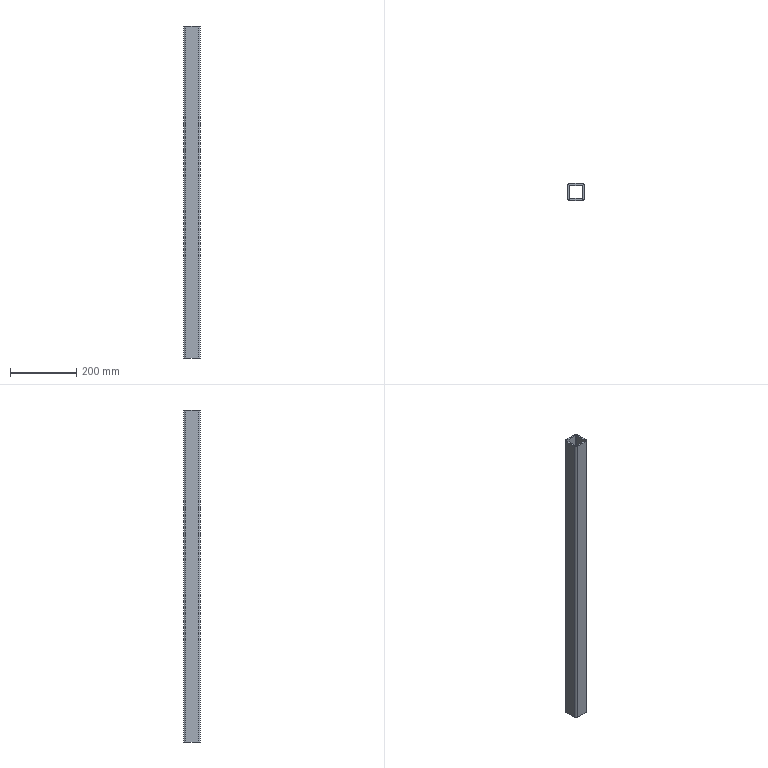Part | SolidWorks | features Extrusion 1 | 1 solid | 18 faces | box 50 x 50 x 1000 mm | volume 869956 mm3 | plane 10 | cylinder 8 | commonest cylinder face diameters 2 x4 12 x4
STEP:
#1=CARTESIAN_POINT('',(0.,6.,1000.));
#2=VERTEX_POINT('',#1);
#3=CARTESIAN_POINT('',(6.,0.,1000.));
#4=VERTEX_POINT('',#3);
#5=CARTESIAN_POINT('',(6.,6.,1000.));
#6=DIRECTION('',(0.,0.,1.));
#7=DIRECTION('',(-1.,0.,0.));
#8=AXIS2_PLACEMENT_3D('',#5,#6,#7);
#9=CIRCLE('',#8,6.);
#10=EDGE_CURVE('',#2,#4,#9,.T.);
#11=ORIENTED_EDGE('',*,*,#10,.T.);
#12=CARTESIAN_POINT('',(44.,0.,1000.));
#13=VERTEX_POINT('',#12);
#14=CARTESIAN_POINT('',(6.,0.,1000.));
#15=DIRECTION('',(1.,0.,0.));
#16=VECTOR('',#15,1000.);
#17=LINE('',#14,#16);
#18=EDGE_CURVE('',#4,#13,#17,.T.);
#19=ORIENTED_EDGE('',*,*,#18,.T.);
#20=CARTESIAN_POINT('',(50.,6.,1000.));
#21=VERTEX_POINT('',#20);
#22=CARTESIAN_POINT('',(44.,6.,1000.));
#23=DIRECTION('',(0.,0.,1.));
#24=DIRECTION('',(1.,0.,0.));
#25=AXIS2_PLACEMENT_3D('',#22,#23,#24);
#26=CIRCLE('',#25,6.);
#27=EDGE_CURVE('',#13,#21,#26,.T.);
#28=ORIENTED_EDGE('',*,*,#27,.T.);
#29=CARTESIAN_POINT('',(50.,44.,1000.));
#30=VERTEX_POINT('',#29);
#31=CARTESIAN_POINT('',(50.,6.,1000.));
#32=DIRECTION('',(0.,1.,0.));
#33=VECTOR('',#32,1000.);
#34=LINE('',#31,#33);
#35=EDGE_CURVE('',#21,#30,#34,.T.);
#36=ORIENTED_EDGE('',*,*,#35,.T.);
#37=CARTESIAN_POINT('',(44.,50.,1000.));
#38=VERTEX_POINT('',#37);
#39=CARTESIAN_POINT('',(44.,44.,1000.));
#40=DIRECTION('',(0.,0.,1.));
#41=DIRECTION('',(-1.,0.,0.));
#42=AXIS2_PLACEMENT_3D('',#39,#40,#41);
#43=CIRCLE('',#42,6.);
#44=EDGE_CURVE('',#30,#38,#43,.T.);
#45=ORIENTED_EDGE('',*,*,#44,.T.);
#46=CARTESIAN_POINT('',(6.,50.,1000.));
#47=VERTEX_POINT('',#46);
#48=CARTESIAN_POINT('',(6.,50.,1000.));
#49=DIRECTION('',(-1.,0.,0.));
#50=VECTOR('',#49,1000.);
#51=LINE('',#48,#50);
#52=EDGE_CURVE('',#38,#47,#51,.T.);
#53=ORIENTED_EDGE('',*,*,#52,.T.);
#54=CARTESIAN_POINT('',(0.,44.,1000.));
#55=VERTEX_POINT('',#54);
#56=CARTESIAN_POINT('',(6.,44.,1000.));
#57=DIRECTION('',(0.,0.,1.));
#58=DIRECTION('',(-1.,0.,0.));
#59=AXIS2_PLACEMENT_3D('',#56,#57,#58);
#60=CIRCLE('',#59,6.);
#61=EDGE_CURVE('',#47,#55,#60,.T.);
#62=ORIENTED_EDGE('',*,*,#61,.T.);
#63=CARTESIAN_POINT('',(0.,6.,1000.));
#64=DIRECTION('',(0.,-1.,0.));
#65=VECTOR('',#64,1000.);
#66=LINE('',#63,#65);
#67=EDGE_CURVE('',#55,#2,#66,.T.);
#68=ORIENTED_EDGE('',*,*,#67,.T.);
#69=EDGE_LOOP('',(#11,#19,#28,#36,#45,#53,#62,#68));
#70=FACE_OUTER_BOUND('',#69,.T.);
#71=CARTESIAN_POINT('',(6.,45.,1000.));
#72=VERTEX_POINT('',#71);
#73=CARTESIAN_POINT('',(5.,44.,1000.));
#74=VERTEX_POINT('',#73);
#75=CARTESIAN_POINT('',(6.,44.,1000.));
#76=DIRECTION('',(0.,0.,1.));
#77=DIRECTION('',(-1.,0.,0.));
#78=AXIS2_PLACEMENT_3D('',#75,#76,#77);
#79=CIRCLE('',#78,1.);
#80=EDGE_CURVE('',#72,#74,#79,.T.);
#81=ORIENTED_EDGE('',*,*,#80,.F.);
#82=CARTESIAN_POINT('',(44.,45.,1000.));
#83=VERTEX_POINT('',#82);
#84=CARTESIAN_POINT('',(6.,45.,1000.));
#85=DIRECTION('',(-1.,0.,0.));
#86=VECTOR('',#85,1000.);
#87=LINE('',#84,#86);
#88=EDGE_CURVE('',#83,#72,#87,.T.);
#89=ORIENTED_EDGE('',*,*,#88,.F.);
#90=CARTESIAN_POINT('',(45.,44.,1000.));
#91=VERTEX_POINT('',#90);
#92=CARTESIAN_POINT('',(44.,44.,1000.));
#93=DIRECTION('',(0.,0.,1.));
#94=DIRECTION('',(-1.,0.,0.));
#95=AXIS2_PLACEMENT_3D('',#92,#93,#94);
#96=CIRCLE('',#95,1.);
#97=EDGE_CURVE('',#91,#83,#96,.T.);
#98=ORIENTED_EDGE('',*,*,#97,.F.);
#99=CARTESIAN_POINT('',(45.,6.,1000.));
#100=VERTEX_POINT('',#99);
#101=CARTESIAN_POINT('',(45.,6.,1000.));
#102=DIRECTION('',(0.,1.,0.));
#103=VECTOR('',#102,1000.);
#104=LINE('',#101,#103);
#105=EDGE_CURVE('',#100,#91,#104,.T.);
#106=ORIENTED_EDGE('',*,*,#105,.F.);
#107=CARTESIAN_POINT('',(44.,5.,1000.));
#108=VERTEX_POINT('',#107);
#109=CARTESIAN_POINT('',(44.,6.,1000.));
#110=DIRECTION('',(0.,0.,1.));
#111=DIRECTION('',(1.,0.,0.));
#112=AXIS2_PLACEMENT_3D('',#109,#110,#111);
#113=CIRCLE('',#112,1.);
#114=EDGE_CURVE('',#108,#100,#113,.T.);
#115=ORIENTED_EDGE('',*,*,#114,.F.);
#116=CARTESIAN_POINT('',(6.,5.,1000.));
#117=VERTEX_POINT('',#116);
#118=CARTESIAN_POINT('',(6.,5.,1000.));
#119=DIRECTION('',(1.,0.,0.));
#120=VECTOR('',#119,1000.);
#121=LINE('',#118,#120);
#122=EDGE_CURVE('',#117,#108,#121,.T.);
#123=ORIENTED_EDGE('',*,*,#122,.F.);
#124=CARTESIAN_POINT('',(5.,6.,1000.));
#125=VERTEX_POINT('',#124);
#126=CARTESIAN_POINT('',(6.,6.,1000.));
#127=DIRECTION('',(0.,0.,1.));
#128=DIRECTION('',(-1.,0.,0.));
#129=AXIS2_PLACEMENT_3D('',#126,#127,#128);
#130=CIRCLE('',#129,1.);
#131=EDGE_CURVE('',#125,#117,#130,.T.);
#132=ORIENTED_EDGE('',*,*,#131,.F.);
#133=CARTESIAN_POINT('',(5.,6.,1000.));
#134=DIRECTION('',(0.,-1.,0.));
#135=VECTOR('',#134,1000.);
#136=LINE('',#133,#135);
#137=EDGE_CURVE('',#74,#125,#136,.T.);
#138=ORIENTED_EDGE('',*,*,#137,.F.);
#139=EDGE_LOOP('',(#81,#89,#98,#106,#115,#123,#132,#138));
#140=FACE_BOUND('',#139,.T.);
#141=CARTESIAN_POINT('',(6.,6.,1000.));
#142=DIRECTION('',(0.,0.,-1.));
#143=DIRECTION('',(-1.,0.,0.));
#144=AXIS2_PLACEMENT_3D('',#141,#142,#143);
#145=PLANE('',#144);
#146=ADVANCED_FACE('',(#70,#140),#145,.F.);
#147=CARTESIAN_POINT('',(0.,6.,0.));
#148=VERTEX_POINT('',#147);
#149=CARTESIAN_POINT('',(6.,0.,0.));
#150=VERTEX_POINT('',#149);
#151=CARTESIAN_POINT('',(6.,6.,0.));
#152=DIRECTION('',(0.,0.,1.));
#153=DIRECTION('',(-1.,0.,0.));
#154=AXIS2_PLACEMENT_3D('',#151,#152,#153);
#155=CIRCLE('',#154,6.);
#156=EDGE_CURVE('',#148,#150,#155,.T.);
#157=ORIENTED_EDGE('',*,*,#156,.F.);
#158=CARTESIAN_POINT('',(0.,44.,0.));
#159=VERTEX_POINT('',#158);
#160=CARTESIAN_POINT('',(0.,6.,0.));
#161=DIRECTION('',(0.,-1.,0.));
#162=VECTOR('',#161,1000.);
#163=LINE('',#160,#162);
#164=EDGE_CURVE('',#159,#148,#163,.T.);
#165=ORIENTED_EDGE('',*,*,#164,.F.);
#166=CARTESIAN_POINT('',(6.,50.,0.));
#167=VERTEX_POINT('',#166);
#168=CARTESIAN_POINT('',(6.,44.,0.));
#169=DIRECTION('',(0.,0.,1.));
#170=DIRECTION('',(-1.,0.,0.));
#171=AXIS2_PLACEMENT_3D('',#168,#169,#170);
#172=CIRCLE('',#171,6.);
#173=EDGE_CURVE('',#167,#159,#172,.T.);
#174=ORIENTED_EDGE('',*,*,#173,.F.);
#175=CARTESIAN_POINT('',(44.,50.,0.));
#176=VERTEX_POINT('',#175);
#177=CARTESIAN_POINT('',(6.,50.,0.));
#178=DIRECTION('',(-1.,0.,0.));
#179=VECTOR('',#178,1000.);
#180=LINE('',#177,#179);
#181=EDGE_CURVE('',#176,#167,#180,.T.);
#182=ORIENTED_EDGE('',*,*,#181,.F.);
#183=CARTESIAN_POINT('',(50.,44.,0.));
#184=VERTEX_POINT('',#183);
#185=CARTESIAN_POINT('',(44.,44.,0.));
#186=DIRECTION('',(0.,0.,1.));
#187=DIRECTION('',(-1.,0.,0.));
#188=AXIS2_PLACEMENT_3D('',#185,#186,#187);
#189=CIRCLE('',#188,6.);
#190=EDGE_CURVE('',#184,#176,#189,.T.);
#191=ORIENTED_EDGE('',*,*,#190,.F.);
#192=CARTESIAN_POINT('',(50.,6.,0.));
#193=VERTEX_POINT('',#192);
#194=CARTESIAN_POINT('',(50.,6.,0.));
#195=DIRECTION('',(0.,1.,0.));
#196=VECTOR('',#195,1000.);
#197=LINE('',#194,#196);
#198=EDGE_CURVE('',#193,#184,#197,.T.);
#199=ORIENTED_EDGE('',*,*,#198,.F.);
#200=CARTESIAN_POINT('',(44.,0.,0.));
#201=VERTEX_POINT('',#200);
#202=CARTESIAN_POINT('',(44.,6.,0.));
#203=DIRECTION('',(0.,0.,1.));
#204=DIRECTION('',(1.,0.,0.));
#205=AXIS2_PLACEMENT_3D('',#202,#203,#204);
#206=CIRCLE('',#205,6.);
#207=EDGE_CURVE('',#201,#193,#206,.T.);
#208=ORIENTED_EDGE('',*,*,#207,.F.);
#209=CARTESIAN_POINT('',(6.,0.,0.));
#210=DIRECTION('',(1.,0.,0.));
#211=VECTOR('',#210,1000.);
#212=LINE('',#209,#211);
#213=EDGE_CURVE('',#150,#201,#212,.T.);
#214=ORIENTED_EDGE('',*,*,#213,.F.);
#215=EDGE_LOOP('',(#157,#165,#174,#182,#191,#199,#208,#214));
#216=FACE_OUTER_BOUND('',#215,.T.);
#217=CARTESIAN_POINT('',(44.,45.,0.));
#218=VERTEX_POINT('',#217);
#219=CARTESIAN_POINT('',(6.,45.,0.));
#220=VERTEX_POINT('',#219);
#221=CARTESIAN_POINT('',(6.,45.,0.));
#222=DIRECTION('',(-1.,0.,0.));
#223=VECTOR('',#222,1000.);
#224=LINE('',#221,#223);
#225=EDGE_CURVE('',#218,#220,#224,.T.);
#226=ORIENTED_EDGE('',*,*,#225,.T.);
#227=CARTESIAN_POINT('',(5.,44.,0.));
#228=VERTEX_POINT('',#227);
#229=CARTESIAN_POINT('',(6.,44.,0.));
#230=DIRECTION('',(0.,0.,1.));
#231=DIRECTION('',(-1.,0.,0.));
#232=AXIS2_PLACEMENT_3D('',#229,#230,#231);
#233=CIRCLE('',#232,1.);
#234=EDGE_CURVE('',#220,#228,#233,.T.);
#235=ORIENTED_EDGE('',*,*,#234,.T.);
#236=CARTESIAN_POINT('',(5.,6.,0.));
#237=VERTEX_POINT('',#236);
#238=CARTESIAN_POINT('',(5.,6.,0.));
#239=DIRECTION('',(0.,-1.,0.));
#240=VECTOR('',#239,1000.);
#241=LINE('',#238,#240);
#242=EDGE_CURVE('',#228,#237,#241,.T.);
#243=ORIENTED_EDGE('',*,*,#242,.T.);
#244=CARTESIAN_POINT('',(6.,5.,0.));
#245=VERTEX_POINT('',#244);
#246=CARTESIAN_POINT('',(6.,6.,0.));
#247=DIRECTION('',(0.,0.,1.));
#248=DIRECTION('',(-1.,0.,0.));
#249=AXIS2_PLACEMENT_3D('',#246,#247,#248);
#250=CIRCLE('',#249,1.);
#251=EDGE_CURVE('',#237,#245,#250,.T.);
#252=ORIENTED_EDGE('',*,*,#251,.T.);
#253=CARTESIAN_POINT('',(44.,5.,0.));
#254=VERTEX_POINT('',#253);
#255=CARTESIAN_POINT('',(6.,5.,0.));
#256=DIRECTION('',(1.,0.,0.));
#257=VECTOR('',#256,1000.);
#258=LINE('',#255,#257);
#259=EDGE_CURVE('',#245,#254,#258,.T.);
#260=ORIENTED_EDGE('',*,*,#259,.T.);
#261=CARTESIAN_POINT('',(45.,6.,0.));
#262=VERTEX_POINT('',#261);
#263=CARTESIAN_POINT('',(44.,6.,0.));
#264=DIRECTION('',(0.,0.,1.));
#265=DIRECTION('',(1.,0.,0.));
#266=AXIS2_PLACEMENT_3D('',#263,#264,#265);
#267=CIRCLE('',#266,1.);
#268=EDGE_CURVE('',#254,#262,#267,.T.);
#269=ORIENTED_EDGE('',*,*,#268,.T.);
#270=CARTESIAN_POINT('',(45.,44.,0.));
#271=VERTEX_POINT('',#270);
#272=CARTESIAN_POINT('',(45.,6.,0.));
#273=DIRECTION('',(0.,1.,0.));
#274=VECTOR('',#273,1000.);
#275=LINE('',#272,#274);
#276=EDGE_CURVE('',#262,#271,#275,.T.);
#277=ORIENTED_EDGE('',*,*,#276,.T.);
#278=CARTESIAN_POINT('',(44.,44.,0.));
#279=DIRECTION('',(0.,0.,1.));
#280=DIRECTION('',(-1.,0.,0.));
#281=AXIS2_PLACEMENT_3D('',#278,#279,#280);
#282=CIRCLE('',#281,1.);
#283=EDGE_CURVE('',#271,#218,#282,.T.);
#284=ORIENTED_EDGE('',*,*,#283,.T.);
#285=EDGE_LOOP('',(#226,#235,#243,#252,#260,#269,#277,#284));
#286=FACE_BOUND('',#285,.T.);
#287=CARTESIAN_POINT('',(6.,6.,0.));
#288=DIRECTION('',(0.,0.,-1.));
#289=DIRECTION('',(-1.,0.,0.));
#290=AXIS2_PLACEMENT_3D('',#287,#288,#289);
#291=PLANE('',#290);
#292=ADVANCED_FACE('',(#216,#286),#291,.T.);
#293=ORIENTED_EDGE('',*,*,#156,.T.);
#294=CARTESIAN_POINT('',(6.,0.,1000.));
#295=DIRECTION('',(0.,0.,-1.));
#296=VECTOR('',#295,1000.);
#297=LINE('',#294,#296);
#298=EDGE_CURVE('',#4,#150,#297,.T.);
#299=ORIENTED_EDGE('',*,*,#298,.F.);
#300=ORIENTED_EDGE('',*,*,#10,.F.);
#301=CARTESIAN_POINT('',(0.,6.,1000.));
#302=DIRECTION('',(0.,0.,-1.));
#303=VECTOR('',#302,1000.);
#304=LINE('',#301,#303);
#305=EDGE_CURVE('',#2,#148,#304,.T.);
#306=ORIENTED_EDGE('',*,*,#305,.T.);
#307=EDGE_LOOP('',(#293,#299,#300,#306));
#308=FACE_OUTER_BOUND('',#307,.T.);
#309=CARTESIAN_POINT('',(6.,6.,1000.));
#310=DIRECTION('',(0.,0.,-1.));
#311=DIRECTION('',(-1.,0.,0.));
#312=AXIS2_PLACEMENT_3D('',#309,#310,#311);
#313=CYLINDRICAL_SURFACE('',#312,6.);
#314=ADVANCED_FACE('',(#308),#313,.T.);
#315=ORIENTED_EDGE('',*,*,#213,.T.);
#316=CARTESIAN_POINT('',(44.,0.,1000.));
#317=DIRECTION('',(0.,0.,-1.));
#318=VECTOR('',#317,1000.);
#319=LINE('',#316,#318);
#320=EDGE_CURVE('',#13,#201,#319,.T.);
#321=ORIENTED_EDGE('',*,*,#320,.F.);
#322=ORIENTED_EDGE('',*,*,#18,.F.);
#323=ORIENTED_EDGE('',*,*,#298,.T.);
#324=EDGE_LOOP('',(#315,#321,#322,#323));
#325=FACE_OUTER_BOUND('',#324,.T.);
#326=CARTESIAN_POINT('',(6.,0.,1000.));
#327=DIRECTION('',(0.,1.,0.));
#328=DIRECTION('',(0.,0.,1.));
#329=AXIS2_PLACEMENT_3D('',#326,#327,#328);
#330=PLANE('',#329);
#331=ADVANCED_FACE('',(#325),#330,.F.);
#332=ORIENTED_EDGE('',*,*,#207,.T.);
#333=CARTESIAN_POINT('',(50.,6.,1000.));
#334=DIRECTION('',(0.,0.,-1.));
#335=VECTOR('',#334,1000.);
#336=LINE('',#333,#335);
#337=EDGE_CURVE('',#21,#193,#336,.T.);
#338=ORIENTED_EDGE('',*,*,#337,.F.);
#339=ORIENTED_EDGE('',*,*,#27,.F.);
#340=ORIENTED_EDGE('',*,*,#320,.T.);
#341=EDGE_LOOP('',(#332,#338,#339,#340));
#342=FACE_OUTER_BOUND('',#341,.T.);
#343=CARTESIAN_POINT('',(44.,6.,1000.));
#344=DIRECTION('',(0.,0.,-1.));
#345=DIRECTION('',(-1.,0.,0.));
#346=AXIS2_PLACEMENT_3D('',#343,#344,#345);
#347=CYLINDRICAL_SURFACE('',#346,6.);
#348=ADVANCED_FACE('',(#342),#347,.T.);
#349=ORIENTED_EDGE('',*,*,#198,.T.);
#350=CARTESIAN_POINT('',(50.,44.,1000.));
#351=DIRECTION('',(0.,0.,-1.));
#352=VECTOR('',#351,1000.);
#353=LINE('',#350,#352);
#354=EDGE_CURVE('',#30,#184,#353,.T.);
#355=ORIENTED_EDGE('',*,*,#354,.F.);
#356=ORIENTED_EDGE('',*,*,#35,.F.);
#357=ORIENTED_EDGE('',*,*,#337,.T.);
#358=EDGE_LOOP('',(#349,#355,#356,#357));
#359=FACE_OUTER_BOUND('',#358,.T.);
#360=CARTESIAN_POINT('',(50.,6.,1000.));
#361=DIRECTION('',(-1.,0.,0.));
#362=DIRECTION('',(0.,0.,1.));
#363=AXIS2_PLACEMENT_3D('',#360,#361,#362);
#364=PLANE('',#363);
#365=ADVANCED_FACE('',(#359),#364,.F.);
#366=ORIENTED_EDGE('',*,*,#190,.T.);
#367=CARTESIAN_POINT('',(44.,50.,1000.));
#368=DIRECTION('',(0.,0.,-1.));
#369=VECTOR('',#368,1000.);
#370=LINE('',#367,#369);
#371=EDGE_CURVE('',#38,#176,#370,.T.);
#372=ORIENTED_EDGE('',*,*,#371,.F.);
#373=ORIENTED_EDGE('',*,*,#44,.F.);
#374=ORIENTED_EDGE('',*,*,#354,.T.);
#375=EDGE_LOOP('',(#366,#372,#373,#374));
#376=FACE_OUTER_BOUND('',#375,.T.);
#377=CARTESIAN_POINT('',(44.,44.,1000.));
#378=DIRECTION('',(0.,0.,-1.));
#379=DIRECTION('',(-1.,0.,0.));
#380=AXIS2_PLACEMENT_3D('',#377,#378,#379);
#381=CYLINDRICAL_SURFACE('',#380,6.);
#382=ADVANCED_FACE('',(#376),#381,.T.);
#383=ORIENTED_EDGE('',*,*,#181,.T.);
#384=CARTESIAN_POINT('',(6.,50.,1000.));
#385=DIRECTION('',(0.,0.,-1.));
#386=VECTOR('',#385,1000.);
#387=LINE('',#384,#386);
#388=EDGE_CURVE('',#47,#167,#387,.T.);
#389=ORIENTED_EDGE('',*,*,#388,.F.);
#390=ORIENTED_EDGE('',*,*,#52,.F.);
#391=ORIENTED_EDGE('',*,*,#371,.T.);
#392=EDGE_LOOP('',(#383,#389,#390,#391));
#393=FACE_OUTER_BOUND('',#392,.T.);
#394=CARTESIAN_POINT('',(6.,50.,1000.));
#395=DIRECTION('',(0.,-1.,0.));
#396=DIRECTION('',(0.,0.,-1.));
#397=AXIS2_PLACEMENT_3D('',#394,#395,#396);
#398=PLANE('',#397);
#399=ADVANCED_FACE('',(#393),#398,.F.);
#400=ORIENTED_EDGE('',*,*,#173,.T.);
#401=CARTESIAN_POINT('',(0.,44.,1000.));
#402=DIRECTION('',(0.,0.,-1.));
#403=VECTOR('',#402,1000.);
#404=LINE('',#401,#403);
#405=EDGE_CURVE('',#55,#159,#404,.T.);
#406=ORIENTED_EDGE('',*,*,#405,.F.);
#407=ORIENTED_EDGE('',*,*,#61,.F.);
#408=ORIENTED_EDGE('',*,*,#388,.T.);
#409=EDGE_LOOP('',(#400,#406,#407,#408));
#410=FACE_OUTER_BOUND('',#409,.T.);
#411=CARTESIAN_POINT('',(6.,44.,1000.));
#412=DIRECTION('',(0.,0.,-1.));
#413=DIRECTION('',(-1.,0.,0.));
#414=AXIS2_PLACEMENT_3D('',#411,#412,#413);
#415=CYLINDRICAL_SURFACE('',#414,6.);
#416=ADVANCED_FACE('',(#410),#415,.T.);
#417=ORIENTED_EDGE('',*,*,#164,.T.);
#418=ORIENTED_EDGE('',*,*,#305,.F.);
#419=ORIENTED_EDGE('',*,*,#67,.F.);
#420=ORIENTED_EDGE('',*,*,#405,.T.);
#421=EDGE_LOOP('',(#417,#418,#419,#420));
#422=FACE_OUTER_BOUND('',#421,.T.);
#423=CARTESIAN_POINT('',(0.,6.,1000.));
#424=DIRECTION('',(1.,0.,0.));
#425=DIRECTION('',(0.,0.,-1.));
#426=AXIS2_PLACEMENT_3D('',#423,#424,#425);
#427=PLANE('',#426);
#428=ADVANCED_FACE('',(#422),#427,.F.);
#429=ORIENTED_EDGE('',*,*,#234,.F.);
#430=CARTESIAN_POINT('',(6.,45.,1000.));
#431=DIRECTION('',(0.,0.,-1.));
#432=VECTOR('',#431,1000.);
#433=LINE('',#430,#432);
#434=EDGE_CURVE('',#72,#220,#433,.T.);
#435=ORIENTED_EDGE('',*,*,#434,.F.);
#436=ORIENTED_EDGE('',*,*,#80,.T.);
#437=CARTESIAN_POINT('',(5.,44.,1000.));
#438=DIRECTION('',(0.,0.,-1.));
#439=VECTOR('',#438,1000.);
#440=LINE('',#437,#439);
#441=EDGE_CURVE('',#74,#228,#440,.T.);
#442=ORIENTED_EDGE('',*,*,#441,.T.);
#443=EDGE_LOOP('',(#429,#435,#436,#442));
#444=FACE_OUTER_BOUND('',#443,.T.);
#445=CARTESIAN_POINT('',(6.,44.,1000.));
#446=DIRECTION('',(0.,0.,-1.));
#447=DIRECTION('',(-1.,0.,0.));
#448=AXIS2_PLACEMENT_3D('',#445,#446,#447);
#449=CYLINDRICAL_SURFACE('',#448,1.);
#450=ADVANCED_FACE('',(#444),#449,.F.);
#451=ORIENTED_EDGE('',*,*,#242,.F.);
#452=ORIENTED_EDGE('',*,*,#441,.F.);
#453=ORIENTED_EDGE('',*,*,#137,.T.);
#454=CARTESIAN_POINT('',(5.,6.,1000.));
#455=DIRECTION('',(0.,0.,-1.));
#456=VECTOR('',#455,1000.);
#457=LINE('',#454,#456);
#458=EDGE_CURVE('',#125,#237,#457,.T.);
#459=ORIENTED_EDGE('',*,*,#458,.T.);
#460=EDGE_LOOP('',(#451,#452,#453,#459));
#461=FACE_OUTER_BOUND('',#460,.T.);
#462=CARTESIAN_POINT('',(5.,6.,1000.));
#463=DIRECTION('',(1.,0.,0.));
#464=DIRECTION('',(0.,1.,0.));
#465=AXIS2_PLACEMENT_3D('',#462,#463,#464);
#466=PLANE('',#465);
#467=ADVANCED_FACE('',(#461),#466,.T.);
#468=ORIENTED_EDGE('',*,*,#251,.F.);
#469=ORIENTED_EDGE('',*,*,#458,.F.);
#470=ORIENTED_EDGE('',*,*,#131,.T.);
#471=CARTESIAN_POINT('',(6.,5.,1000.));
#472=DIRECTION('',(0.,0.,-1.));
#473=VECTOR('',#472,1000.);
#474=LINE('',#471,#473);
#475=EDGE_CURVE('',#117,#245,#474,.T.);
#476=ORIENTED_EDGE('',*,*,#475,.T.);
#477=EDGE_LOOP('',(#468,#469,#470,#476));
#478=FACE_OUTER_BOUND('',#477,.T.);
#479=CARTESIAN_POINT('',(6.,6.,1000.));
#480=DIRECTION('',(0.,0.,-1.));
#481=DIRECTION('',(-1.,0.,0.));
#482=AXIS2_PLACEMENT_3D('',#479,#480,#481);
#483=CYLINDRICAL_SURFACE('',#482,1.);
#484=ADVANCED_FACE('',(#478),#483,.F.);
#485=ORIENTED_EDGE('',*,*,#259,.F.);
#486=ORIENTED_EDGE('',*,*,#475,.F.);
#487=ORIENTED_EDGE('',*,*,#122,.T.);
#488=CARTESIAN_POINT('',(44.,5.,1000.));
#489=DIRECTION('',(0.,0.,-1.));
#490=VECTOR('',#489,1000.);
#491=LINE('',#488,#490);
#492=EDGE_CURVE('',#108,#254,#491,.T.);
#493=ORIENTED_EDGE('',*,*,#492,.T.);
#494=EDGE_LOOP('',(#485,#486,#487,#493));
#495=FACE_OUTER_BOUND('',#494,.T.);
#496=CARTESIAN_POINT('',(6.,5.,1000.));
#497=DIRECTION('',(0.,1.,0.));
#498=DIRECTION('',(-1.,0.,0.));
#499=AXIS2_PLACEMENT_3D('',#496,#497,#498);
#500=PLANE('',#499);
#501=ADVANCED_FACE('',(#495),#500,.T.);
#502=ORIENTED_EDGE('',*,*,#268,.F.);
#503=ORIENTED_EDGE('',*,*,#492,.F.);
#504=ORIENTED_EDGE('',*,*,#114,.T.);
#505=CARTESIAN_POINT('',(45.,6.,1000.));
#506=DIRECTION('',(0.,0.,-1.));
#507=VECTOR('',#506,1000.);
#508=LINE('',#505,#507);
#509=EDGE_CURVE('',#100,#262,#508,.T.);
#510=ORIENTED_EDGE('',*,*,#509,.T.);
#511=EDGE_LOOP('',(#502,#503,#504,#510));
#512=FACE_OUTER_BOUND('',#511,.T.);
#513=CARTESIAN_POINT('',(44.,6.,1000.));
#514=DIRECTION('',(0.,0.,-1.));
#515=DIRECTION('',(-1.,0.,0.));
#516=AXIS2_PLACEMENT_3D('',#513,#514,#515);
#517=CYLINDRICAL_SURFACE('',#516,1.);
#518=ADVANCED_FACE('',(#512),#517,.F.);
#519=ORIENTED_EDGE('',*,*,#276,.F.);
#520=ORIENTED_EDGE('',*,*,#509,.F.);
#521=ORIENTED_EDGE('',*,*,#105,.T.);
#522=CARTESIAN_POINT('',(45.,44.,1000.));
#523=DIRECTION('',(0.,0.,-1.));
#524=VECTOR('',#523,1000.);
#525=LINE('',#522,#524);
#526=EDGE_CURVE('',#91,#271,#525,.T.);
#527=ORIENTED_EDGE('',*,*,#526,.T.);
#528=EDGE_LOOP('',(#519,#520,#521,#527));
#529=FACE_OUTER_BOUND('',#528,.T.);
#530=CARTESIAN_POINT('',(45.,6.,1000.));
#531=DIRECTION('',(-1.,0.,0.));
#532=DIRECTION('',(0.,0.,1.));
#533=AXIS2_PLACEMENT_3D('',#530,#531,#532);
#534=PLANE('',#533);
#535=ADVANCED_FACE('',(#529),#534,.T.);
#536=ORIENTED_EDGE('',*,*,#283,.F.);
#537=ORIENTED_EDGE('',*,*,#526,.F.);
#538=ORIENTED_EDGE('',*,*,#97,.T.);
#539=CARTESIAN_POINT('',(44.,45.,1000.));
#540=DIRECTION('',(0.,0.,-1.));
#541=VECTOR('',#540,1000.);
#542=LINE('',#539,#541);
#543=EDGE_CURVE('',#83,#218,#542,.T.);
#544=ORIENTED_EDGE('',*,*,#543,.T.);
#545=EDGE_LOOP('',(#536,#537,#538,#544));
#546=FACE_OUTER_BOUND('',#545,.T.);
#547=CARTESIAN_POINT('',(44.,44.,1000.));
#548=DIRECTION('',(0.,0.,-1.));
#549=DIRECTION('',(-1.,0.,0.));
#550=AXIS2_PLACEMENT_3D('',#547,#548,#549);
#551=CYLINDRICAL_SURFACE('',#550,1.);
#552=ADVANCED_FACE('',(#546),#551,.F.);
#553=ORIENTED_EDGE('',*,*,#225,.F.);
#554=ORIENTED_EDGE('',*,*,#543,.F.);
#555=ORIENTED_EDGE('',*,*,#88,.T.);
#556=ORIENTED_EDGE('',*,*,#434,.T.);
#557=EDGE_LOOP('',(#553,#554,#555,#556));
#558=FACE_OUTER_BOUND('',#557,.T.);
#559=CARTESIAN_POINT('',(6.,45.,1000.));
#560=DIRECTION('',(0.,-1.,0.));
#561=DIRECTION('',(0.,0.,-1.));
#562=AXIS2_PLACEMENT_3D('',#559,#560,#561);
#563=PLANE('',#562);
#564=ADVANCED_FACE('',(#558),#563,.T.);
#565=CLOSED_SHELL('',(#146,#292,#314,#331,#348,#365,#382,#399,#416,#428,#450,#467,#484,#501,#518,#535,#552,#564));
#566=MANIFOLD_SOLID_BREP('',#565);
#567=CARTESIAN_POINT('',(0.,0.,0.));
#568=DIRECTION('',(0.,0.,1.));
#569=DIRECTION('',(1.,0.,0.));
#570=AXIS2_PLACEMENT_3D('',#567,#568,#569);
#571=(LENGTH_UNIT()NAMED_UNIT(*)SI_UNIT(.MILLI.,.METRE.));
#572=UNCERTAINTY_MEASURE_WITH_UNIT(LENGTH_MEASURE(0.00001),#571,'','');
#573=(NAMED_UNIT(*)PLANE_ANGLE_UNIT()SI_UNIT($,.RADIAN.));
#574=(NAMED_UNIT(*)SI_UNIT($,.STERADIAN.)SOLID_ANGLE_UNIT());
#575=(GEOMETRIC_REPRESENTATION_CONTEXT(3)GLOBAL_UNCERTAINTY_ASSIGNED_CONTEXT((#572))GLOBAL_UNIT_ASSIGNED_CONTEXT((#571,#573,#574))REPRESENTATION_CONTEXT('',''));
#576=ADVANCED_BREP_SHAPE_REPRESENTATION('',(#566,#570),#575);